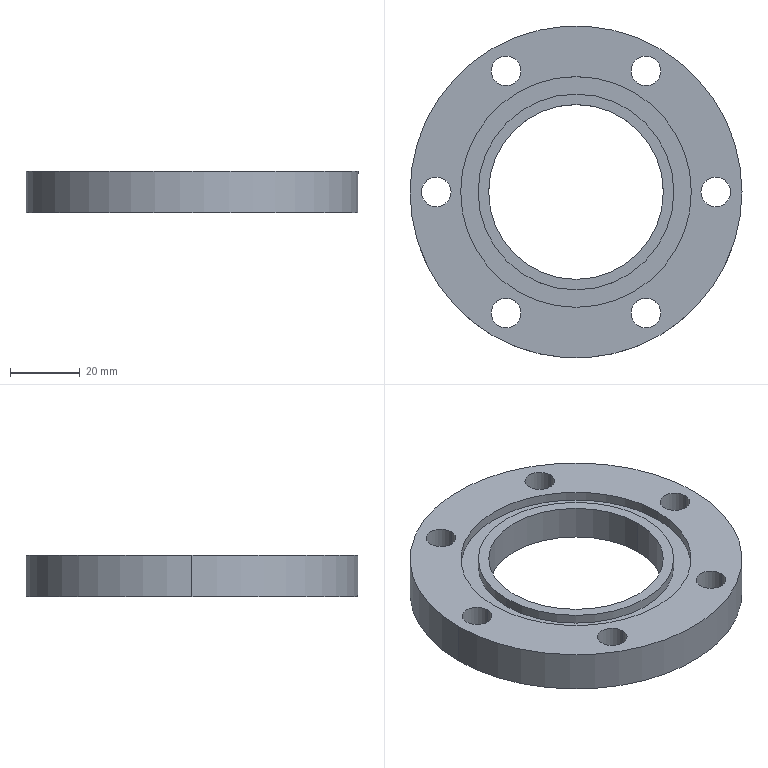Part | SolidWorks | features ICE 2, CirPattern 1, FlatPattern 1, HoleWzd 1, SMBaseFlange 1, SheetMetal 1 | 1 solid | 27 faces | box 95 x 95 x 12 mm | volume 53096 mm3 | cylinder 22 | plane 5 | commonest cylinder face diameters 8.5 x12 50 x2 56 x2 60 x2 66 x2 95 x2
STEP:
#1=CARTESIAN_POINT('',(15.75,-34.641,-12.));
#2=VERTEX_POINT('',#1);
#3=CARTESIAN_POINT('',(24.25,-34.641,-12.));
#4=VERTEX_POINT('',#3);
#5=CARTESIAN_POINT('',(20.,-34.641,-12.));
#6=DIRECTION('',(0.,0.,1.));
#7=DIRECTION('',(1.,0.,0.));
#8=AXIS2_PLACEMENT_3D('',#5,#6,#7);
#9=CIRCLE('',#8,4.25);
#10=EDGE_CURVE('',#2,#4,#9,.T.);
#11=ORIENTED_EDGE('',*,*,#10,.F.);
#12=CARTESIAN_POINT('',(15.75,-34.641,0.));
#13=VERTEX_POINT('',#12);
#14=CARTESIAN_POINT('',(15.75,-34.641,0.));
#15=DIRECTION('',(0.,0.,1.));
#16=VECTOR('',#15,1000.);
#17=LINE('',#14,#16);
#18=EDGE_CURVE('',#2,#13,#17,.T.);
#19=ORIENTED_EDGE('',*,*,#18,.T.);
#20=CARTESIAN_POINT('',(24.25,-34.641,0.));
#21=VERTEX_POINT('',#20);
#22=CARTESIAN_POINT('',(20.,-34.641,0.));
#23=DIRECTION('',(0.,0.,1.));
#24=DIRECTION('',(1.,0.,0.));
#25=AXIS2_PLACEMENT_3D('',#22,#23,#24);
#26=CIRCLE('',#25,4.25);
#27=EDGE_CURVE('',#13,#21,#26,.T.);
#28=ORIENTED_EDGE('',*,*,#27,.T.);
#29=CARTESIAN_POINT('',(24.25,-34.641,0.));
#30=DIRECTION('',(0.,0.,1.));
#31=VECTOR('',#30,1000.);
#32=LINE('',#29,#31);
#33=EDGE_CURVE('',#4,#21,#32,.T.);
#34=ORIENTED_EDGE('',*,*,#33,.F.);
#35=EDGE_LOOP('',(#11,#19,#28,#34));
#36=FACE_OUTER_BOUND('',#35,.T.);
#37=CARTESIAN_POINT('',(20.,-34.641,0.));
#38=DIRECTION('',(0.,0.,1.));
#39=DIRECTION('',(1.,0.,0.));
#40=AXIS2_PLACEMENT_3D('',#37,#38,#39);
#41=CYLINDRICAL_SURFACE('',#40,4.25);
#42=ADVANCED_FACE('',(#36),#41,.F.);
#43=CARTESIAN_POINT('',(-24.25,-34.641,-12.));
#44=VERTEX_POINT('',#43);
#45=CARTESIAN_POINT('',(-15.75,-34.641,-12.));
#46=VERTEX_POINT('',#45);
#47=CARTESIAN_POINT('',(-20.,-34.641,-12.));
#48=DIRECTION('',(0.,0.,1.));
#49=DIRECTION('',(1.,0.,0.));
#50=AXIS2_PLACEMENT_3D('',#47,#48,#49);
#51=CIRCLE('',#50,4.25);
#52=EDGE_CURVE('',#44,#46,#51,.T.);
#53=ORIENTED_EDGE('',*,*,#52,.F.);
#54=CARTESIAN_POINT('',(-24.25,-34.641,0.));
#55=VERTEX_POINT('',#54);
#56=CARTESIAN_POINT('',(-24.25,-34.641,0.));
#57=DIRECTION('',(0.,0.,1.));
#58=VECTOR('',#57,1000.);
#59=LINE('',#56,#58);
#60=EDGE_CURVE('',#44,#55,#59,.T.);
#61=ORIENTED_EDGE('',*,*,#60,.T.);
#62=CARTESIAN_POINT('',(-15.75,-34.641,0.));
#63=VERTEX_POINT('',#62);
#64=CARTESIAN_POINT('',(-20.,-34.641,0.));
#65=DIRECTION('',(0.,0.,1.));
#66=DIRECTION('',(1.,0.,0.));
#67=AXIS2_PLACEMENT_3D('',#64,#65,#66);
#68=CIRCLE('',#67,4.25);
#69=EDGE_CURVE('',#55,#63,#68,.T.);
#70=ORIENTED_EDGE('',*,*,#69,.T.);
#71=CARTESIAN_POINT('',(-15.75,-34.641,0.));
#72=DIRECTION('',(0.,0.,1.));
#73=VECTOR('',#72,1000.);
#74=LINE('',#71,#73);
#75=EDGE_CURVE('',#46,#63,#74,.T.);
#76=ORIENTED_EDGE('',*,*,#75,.F.);
#77=EDGE_LOOP('',(#53,#61,#70,#76));
#78=FACE_OUTER_BOUND('',#77,.T.);
#79=CARTESIAN_POINT('',(-20.,-34.641,0.));
#80=DIRECTION('',(0.,0.,1.));
#81=DIRECTION('',(1.,0.,0.));
#82=AXIS2_PLACEMENT_3D('',#79,#80,#81);
#83=CYLINDRICAL_SURFACE('',#82,4.25);
#84=ADVANCED_FACE('',(#78),#83,.F.);
#85=CARTESIAN_POINT('',(-44.25,0.,-12.));
#86=VERTEX_POINT('',#85);
#87=CARTESIAN_POINT('',(-35.75,0.,-12.));
#88=VERTEX_POINT('',#87);
#89=CARTESIAN_POINT('',(-40.,0.,-12.));
#90=DIRECTION('',(0.,0.,1.));
#91=DIRECTION('',(1.,0.,0.));
#92=AXIS2_PLACEMENT_3D('',#89,#90,#91);
#93=CIRCLE('',#92,4.25);
#94=EDGE_CURVE('',#86,#88,#93,.T.);
#95=ORIENTED_EDGE('',*,*,#94,.F.);
#96=CARTESIAN_POINT('',(-44.25,0.,0.));
#97=VERTEX_POINT('',#96);
#98=CARTESIAN_POINT('',(-44.25,0.,0.));
#99=DIRECTION('',(0.,0.,1.));
#100=VECTOR('',#99,1000.);
#101=LINE('',#98,#100);
#102=EDGE_CURVE('',#86,#97,#101,.T.);
#103=ORIENTED_EDGE('',*,*,#102,.T.);
#104=CARTESIAN_POINT('',(-35.75,0.,0.));
#105=VERTEX_POINT('',#104);
#106=CARTESIAN_POINT('',(-40.,0.,0.));
#107=DIRECTION('',(0.,0.,1.));
#108=DIRECTION('',(1.,0.,0.));
#109=AXIS2_PLACEMENT_3D('',#106,#107,#108);
#110=CIRCLE('',#109,4.25);
#111=EDGE_CURVE('',#97,#105,#110,.T.);
#112=ORIENTED_EDGE('',*,*,#111,.T.);
#113=CARTESIAN_POINT('',(-35.75,0.,0.));
#114=DIRECTION('',(0.,0.,1.));
#115=VECTOR('',#114,1000.);
#116=LINE('',#113,#115);
#117=EDGE_CURVE('',#88,#105,#116,.T.);
#118=ORIENTED_EDGE('',*,*,#117,.F.);
#119=EDGE_LOOP('',(#95,#103,#112,#118));
#120=FACE_OUTER_BOUND('',#119,.T.);
#121=CARTESIAN_POINT('',(-40.,0.,0.));
#122=DIRECTION('',(0.,0.,1.));
#123=DIRECTION('',(1.,0.,0.));
#124=AXIS2_PLACEMENT_3D('',#121,#122,#123);
#125=CYLINDRICAL_SURFACE('',#124,4.25);
#126=ADVANCED_FACE('',(#120),#125,.F.);
#127=CARTESIAN_POINT('',(-24.25,34.641,-12.));
#128=VERTEX_POINT('',#127);
#129=CARTESIAN_POINT('',(-15.75,34.641,-12.));
#130=VERTEX_POINT('',#129);
#131=CARTESIAN_POINT('',(-20.,34.641,-12.));
#132=DIRECTION('',(0.,0.,1.));
#133=DIRECTION('',(1.,0.,0.));
#134=AXIS2_PLACEMENT_3D('',#131,#132,#133);
#135=CIRCLE('',#134,4.25);
#136=EDGE_CURVE('',#128,#130,#135,.T.);
#137=ORIENTED_EDGE('',*,*,#136,.F.);
#138=CARTESIAN_POINT('',(-24.25,34.641,0.));
#139=VERTEX_POINT('',#138);
#140=CARTESIAN_POINT('',(-24.25,34.641,0.));
#141=DIRECTION('',(0.,0.,1.));
#142=VECTOR('',#141,1000.);
#143=LINE('',#140,#142);
#144=EDGE_CURVE('',#128,#139,#143,.T.);
#145=ORIENTED_EDGE('',*,*,#144,.T.);
#146=CARTESIAN_POINT('',(-15.75,34.641,0.));
#147=VERTEX_POINT('',#146);
#148=CARTESIAN_POINT('',(-20.,34.641,0.));
#149=DIRECTION('',(0.,0.,1.));
#150=DIRECTION('',(1.,0.,0.));
#151=AXIS2_PLACEMENT_3D('',#148,#149,#150);
#152=CIRCLE('',#151,4.25);
#153=EDGE_CURVE('',#139,#147,#152,.T.);
#154=ORIENTED_EDGE('',*,*,#153,.T.);
#155=CARTESIAN_POINT('',(-15.75,34.641,0.));
#156=DIRECTION('',(0.,0.,1.));
#157=VECTOR('',#156,1000.);
#158=LINE('',#155,#157);
#159=EDGE_CURVE('',#130,#147,#158,.T.);
#160=ORIENTED_EDGE('',*,*,#159,.F.);
#161=EDGE_LOOP('',(#137,#145,#154,#160));
#162=FACE_OUTER_BOUND('',#161,.T.);
#163=CARTESIAN_POINT('',(-20.,34.641,0.));
#164=DIRECTION('',(0.,0.,1.));
#165=DIRECTION('',(1.,0.,0.));
#166=AXIS2_PLACEMENT_3D('',#163,#164,#165);
#167=CYLINDRICAL_SURFACE('',#166,4.25);
#168=ADVANCED_FACE('',(#162),#167,.F.);
#169=CARTESIAN_POINT('',(15.75,34.641,-12.));
#170=VERTEX_POINT('',#169);
#171=CARTESIAN_POINT('',(24.25,34.641,-12.));
#172=VERTEX_POINT('',#171);
#173=CARTESIAN_POINT('',(20.,34.641,-12.));
#174=DIRECTION('',(0.,0.,1.));
#175=DIRECTION('',(1.,0.,0.));
#176=AXIS2_PLACEMENT_3D('',#173,#174,#175);
#177=CIRCLE('',#176,4.25);
#178=EDGE_CURVE('',#170,#172,#177,.T.);
#179=ORIENTED_EDGE('',*,*,#178,.F.);
#180=CARTESIAN_POINT('',(15.75,34.641,0.));
#181=VERTEX_POINT('',#180);
#182=CARTESIAN_POINT('',(15.75,34.641,0.));
#183=DIRECTION('',(0.,0.,1.));
#184=VECTOR('',#183,1000.);
#185=LINE('',#182,#184);
#186=EDGE_CURVE('',#170,#181,#185,.T.);
#187=ORIENTED_EDGE('',*,*,#186,.T.);
#188=CARTESIAN_POINT('',(24.25,34.641,0.));
#189=VERTEX_POINT('',#188);
#190=CARTESIAN_POINT('',(20.,34.641,0.));
#191=DIRECTION('',(0.,0.,1.));
#192=DIRECTION('',(1.,0.,0.));
#193=AXIS2_PLACEMENT_3D('',#190,#191,#192);
#194=CIRCLE('',#193,4.25);
#195=EDGE_CURVE('',#181,#189,#194,.T.);
#196=ORIENTED_EDGE('',*,*,#195,.T.);
#197=CARTESIAN_POINT('',(24.25,34.641,0.));
#198=DIRECTION('',(0.,0.,1.));
#199=VECTOR('',#198,1000.);
#200=LINE('',#197,#199);
#201=EDGE_CURVE('',#172,#189,#200,.T.);
#202=ORIENTED_EDGE('',*,*,#201,.F.);
#203=EDGE_LOOP('',(#179,#187,#196,#202));
#204=FACE_OUTER_BOUND('',#203,.T.);
#205=CARTESIAN_POINT('',(20.,34.641,0.));
#206=DIRECTION('',(0.,0.,1.));
#207=DIRECTION('',(1.,0.,0.));
#208=AXIS2_PLACEMENT_3D('',#205,#206,#207);
#209=CYLINDRICAL_SURFACE('',#208,4.25);
#210=ADVANCED_FACE('',(#204),#209,.F.);
#211=CARTESIAN_POINT('',(35.75,0.,-12.));
#212=VERTEX_POINT('',#211);
#213=CARTESIAN_POINT('',(44.25,0.,-12.));
#214=VERTEX_POINT('',#213);
#215=CARTESIAN_POINT('',(40.,0.,-12.));
#216=DIRECTION('',(0.,0.,1.));
#217=DIRECTION('',(1.,0.,0.));
#218=AXIS2_PLACEMENT_3D('',#215,#216,#217);
#219=CIRCLE('',#218,4.25);
#220=EDGE_CURVE('',#212,#214,#219,.T.);
#221=ORIENTED_EDGE('',*,*,#220,.F.);
#222=CARTESIAN_POINT('',(35.75,0.,0.));
#223=VERTEX_POINT('',#222);
#224=CARTESIAN_POINT('',(35.75,0.,0.));
#225=DIRECTION('',(0.,0.,1.));
#226=VECTOR('',#225,1000.);
#227=LINE('',#224,#226);
#228=EDGE_CURVE('',#212,#223,#227,.T.);
#229=ORIENTED_EDGE('',*,*,#228,.T.);
#230=CARTESIAN_POINT('',(44.25,0.,0.));
#231=VERTEX_POINT('',#230);
#232=CARTESIAN_POINT('',(40.,0.,0.));
#233=DIRECTION('',(0.,0.,1.));
#234=DIRECTION('',(1.,0.,0.));
#235=AXIS2_PLACEMENT_3D('',#232,#233,#234);
#236=CIRCLE('',#235,4.25);
#237=EDGE_CURVE('',#223,#231,#236,.T.);
#238=ORIENTED_EDGE('',*,*,#237,.T.);
#239=CARTESIAN_POINT('',(44.25,0.,0.));
#240=DIRECTION('',(0.,0.,1.));
#241=VECTOR('',#240,1000.);
#242=LINE('',#239,#241);
#243=EDGE_CURVE('',#214,#231,#242,.T.);
#244=ORIENTED_EDGE('',*,*,#243,.F.);
#245=EDGE_LOOP('',(#221,#229,#238,#244));
#246=FACE_OUTER_BOUND('',#245,.T.);
#247=CARTESIAN_POINT('',(40.,0.,0.));
#248=DIRECTION('',(0.,0.,1.));
#249=DIRECTION('',(1.,0.,0.));
#250=AXIS2_PLACEMENT_3D('',#247,#248,#249);
#251=CYLINDRICAL_SURFACE('',#250,4.25);
#252=ADVANCED_FACE('',(#246),#251,.F.);
#253=CARTESIAN_POINT('',(30.,0.,-12.));
#254=VERTEX_POINT('',#253);
#255=CARTESIAN_POINT('',(-30.,0.,-12.));
#256=VERTEX_POINT('',#255);
#257=CARTESIAN_POINT('',(0.,0.,-12.));
#258=DIRECTION('',(0.,0.,-1.));
#259=DIRECTION('',(-1.,0.,0.));
#260=AXIS2_PLACEMENT_3D('',#257,#258,#259);
#261=CIRCLE('',#260,30.);
#262=EDGE_CURVE('',#254,#256,#261,.T.);
#263=ORIENTED_EDGE('',*,*,#262,.T.);
#264=CARTESIAN_POINT('',(-30.,0.,-10.));
#265=VERTEX_POINT('',#264);
#266=CARTESIAN_POINT('',(-30.,0.,-12.));
#267=DIRECTION('',(0.,0.,1.));
#268=VECTOR('',#267,1000.);
#269=LINE('',#266,#268);
#270=EDGE_CURVE('',#256,#265,#269,.T.);
#271=ORIENTED_EDGE('',*,*,#270,.T.);
#272=CARTESIAN_POINT('',(30.,0.,-10.));
#273=VERTEX_POINT('',#272);
#274=CARTESIAN_POINT('',(0.,0.,-10.));
#275=DIRECTION('',(0.,0.,-1.));
#276=DIRECTION('',(-1.,0.,0.));
#277=AXIS2_PLACEMENT_3D('',#274,#275,#276);
#278=CIRCLE('',#277,30.);
#279=EDGE_CURVE('',#273,#265,#278,.T.);
#280=ORIENTED_EDGE('',*,*,#279,.F.);
#281=CARTESIAN_POINT('',(30.,0.,-12.));
#282=DIRECTION('',(0.,0.,1.));
#283=VECTOR('',#282,1000.);
#284=LINE('',#281,#283);
#285=EDGE_CURVE('',#254,#273,#284,.T.);
#286=ORIENTED_EDGE('',*,*,#285,.F.);
#287=EDGE_LOOP('',(#263,#271,#280,#286));
#288=FACE_OUTER_BOUND('',#287,.T.);
#289=CARTESIAN_POINT('',(0.,0.,-12.));
#290=DIRECTION('',(0.,0.,1.));
#291=DIRECTION('',(1.,0.,0.));
#292=AXIS2_PLACEMENT_3D('',#289,#290,#291);
#293=CYLINDRICAL_SURFACE('',#292,30.);
#294=ADVANCED_FACE('',(#288),#293,.F.);
#295=CARTESIAN_POINT('',(28.,0.,-2.7));
#296=VERTEX_POINT('',#295);
#297=CARTESIAN_POINT('',(-28.,0.,-2.7));
#298=VERTEX_POINT('',#297);
#299=CARTESIAN_POINT('',(0.,0.,-2.7));
#300=DIRECTION('',(0.,0.,1.));
#301=DIRECTION('',(1.,0.,0.));
#302=AXIS2_PLACEMENT_3D('',#299,#300,#301);
#303=CIRCLE('',#302,28.);
#304=EDGE_CURVE('',#296,#298,#303,.T.);
#305=ORIENTED_EDGE('',*,*,#304,.T.);
#306=CARTESIAN_POINT('',(-28.,0.,0.));
#307=VERTEX_POINT('',#306);
#308=CARTESIAN_POINT('',(-28.,0.,-2.7));
#309=DIRECTION('',(0.,0.,1.));
#310=VECTOR('',#309,1000.);
#311=LINE('',#308,#310);
#312=EDGE_CURVE('',#298,#307,#311,.T.);
#313=ORIENTED_EDGE('',*,*,#312,.T.);
#314=CARTESIAN_POINT('',(28.,0.,0.));
#315=VERTEX_POINT('',#314);
#316=CARTESIAN_POINT('',(0.,0.,0.));
#317=DIRECTION('',(0.,0.,1.));
#318=DIRECTION('',(1.,0.,0.));
#319=AXIS2_PLACEMENT_3D('',#316,#317,#318);
#320=CIRCLE('',#319,28.);
#321=EDGE_CURVE('',#315,#307,#320,.T.);
#322=ORIENTED_EDGE('',*,*,#321,.F.);
#323=CARTESIAN_POINT('',(28.,0.,-2.7));
#324=DIRECTION('',(0.,0.,1.));
#325=VECTOR('',#324,1000.);
#326=LINE('',#323,#325);
#327=EDGE_CURVE('',#296,#315,#326,.T.);
#328=ORIENTED_EDGE('',*,*,#327,.F.);
#329=EDGE_LOOP('',(#305,#313,#322,#328));
#330=FACE_OUTER_BOUND('',#329,.T.);
#331=CARTESIAN_POINT('',(0.,0.,-2.7));
#332=DIRECTION('',(0.,0.,1.));
#333=DIRECTION('',(1.,0.,0.));
#334=AXIS2_PLACEMENT_3D('',#331,#332,#333);
#335=CYLINDRICAL_SURFACE('',#334,28.);
#336=ADVANCED_FACE('',(#330),#335,.T.);
#337=CARTESIAN_POINT('',(-33.,0.,-2.7));
#338=VERTEX_POINT('',#337);
#339=CARTESIAN_POINT('',(33.,0.,-2.7));
#340=VERTEX_POINT('',#339);
#341=CARTESIAN_POINT('',(0.,0.,-2.7));
#342=DIRECTION('',(0.,0.,1.));
#343=DIRECTION('',(1.,0.,0.));
#344=AXIS2_PLACEMENT_3D('',#341,#342,#343);
#345=CIRCLE('',#344,33.);
#346=EDGE_CURVE('',#338,#340,#345,.T.);
#347=ORIENTED_EDGE('',*,*,#346,.F.);
#348=CARTESIAN_POINT('',(-33.,0.,0.));
#349=VERTEX_POINT('',#348);
#350=CARTESIAN_POINT('',(-33.,0.,-2.7));
#351=DIRECTION('',(0.,0.,1.));
#352=VECTOR('',#351,1000.);
#353=LINE('',#350,#352);
#354=EDGE_CURVE('',#338,#349,#353,.T.);
#355=ORIENTED_EDGE('',*,*,#354,.T.);
#356=CARTESIAN_POINT('',(33.,0.,0.));
#357=VERTEX_POINT('',#356);
#358=CARTESIAN_POINT('',(0.,0.,0.));
#359=DIRECTION('',(0.,0.,1.));
#360=DIRECTION('',(1.,0.,0.));
#361=AXIS2_PLACEMENT_3D('',#358,#359,#360);
#362=CIRCLE('',#361,33.);
#363=EDGE_CURVE('',#349,#357,#362,.T.);
#364=ORIENTED_EDGE('',*,*,#363,.T.);
#365=CARTESIAN_POINT('',(33.,0.,-2.7));
#366=DIRECTION('',(0.,0.,1.));
#367=VECTOR('',#366,1000.);
#368=LINE('',#365,#367);
#369=EDGE_CURVE('',#340,#357,#368,.T.);
#370=ORIENTED_EDGE('',*,*,#369,.F.);
#371=EDGE_LOOP('',(#347,#355,#364,#370));
#372=FACE_OUTER_BOUND('',#371,.T.);
#373=CARTESIAN_POINT('',(0.,0.,-2.7));
#374=DIRECTION('',(0.,0.,1.));
#375=DIRECTION('',(1.,0.,0.));
#376=AXIS2_PLACEMENT_3D('',#373,#374,#375);
#377=CYLINDRICAL_SURFACE('',#376,33.);
#378=ADVANCED_FACE('',(#372),#377,.F.);
#379=CARTESIAN_POINT('',(-25.,0.,-10.));
#380=VERTEX_POINT('',#379);
#381=CARTESIAN_POINT('',(25.,0.,-10.));
#382=VERTEX_POINT('',#381);
#383=CARTESIAN_POINT('',(0.,0.,-10.));
#384=DIRECTION('',(0.,0.,1.));
#385=DIRECTION('',(1.,0.,0.));
#386=AXIS2_PLACEMENT_3D('',#383,#384,#385);
#387=CIRCLE('',#386,25.);
#388=EDGE_CURVE('',#380,#382,#387,.T.);
#389=ORIENTED_EDGE('',*,*,#388,.F.);
#390=CARTESIAN_POINT('',(-25.,0.,0.));
#391=VERTEX_POINT('',#390);
#392=CARTESIAN_POINT('',(-25.,0.,-10.));
#393=DIRECTION('',(0.,0.,1.));
#394=VECTOR('',#393,1000.);
#395=LINE('',#392,#394);
#396=EDGE_CURVE('',#380,#391,#395,.T.);
#397=ORIENTED_EDGE('',*,*,#396,.T.);
#398=CARTESIAN_POINT('',(25.,0.,0.));
#399=VERTEX_POINT('',#398);
#400=CARTESIAN_POINT('',(0.,0.,0.));
#401=DIRECTION('',(0.,0.,1.));
#402=DIRECTION('',(1.,0.,0.));
#403=AXIS2_PLACEMENT_3D('',#400,#401,#402);
#404=CIRCLE('',#403,25.);
#405=EDGE_CURVE('',#391,#399,#404,.T.);
#406=ORIENTED_EDGE('',*,*,#405,.T.);
#407=CARTESIAN_POINT('',(25.,0.,-10.));
#408=DIRECTION('',(0.,0.,1.));
#409=VECTOR('',#408,1000.);
#410=LINE('',#407,#409);
#411=EDGE_CURVE('',#382,#399,#410,.T.);
#412=ORIENTED_EDGE('',*,*,#411,.F.);
#413=EDGE_LOOP('',(#389,#397,#406,#412));
#414=FACE_OUTER_BOUND('',#413,.T.);
#415=CARTESIAN_POINT('',(0.,0.,-10.));
#416=DIRECTION('',(0.,0.,1.));
#417=DIRECTION('',(1.,0.,0.));
#418=AXIS2_PLACEMENT_3D('',#415,#416,#417);
#419=CYLINDRICAL_SURFACE('',#418,25.);
#420=ADVANCED_FACE('',(#414),#419,.F.);
#421=CARTESIAN_POINT('',(-47.5,0.,-12.));
#422=VERTEX_POINT('',#421);
#423=CARTESIAN_POINT('',(47.5,0.,-12.));
#424=VERTEX_POINT('',#423);
#425=CARTESIAN_POINT('',(0.,0.,-12.));
#426=DIRECTION('',(0.,0.,-1.));
#427=DIRECTION('',(-1.,0.,0.));
#428=AXIS2_PLACEMENT_3D('',#425,#426,#427);
#429=CIRCLE('',#428,47.5);
#430=EDGE_CURVE('',#422,#424,#429,.T.);
#431=ORIENTED_EDGE('',*,*,#430,.F.);
#432=CARTESIAN_POINT('',(-47.5,0.,0.));
#433=VERTEX_POINT('',#432);
#434=CARTESIAN_POINT('',(-47.5,0.,-10.));
#435=DIRECTION('',(0.,0.,1.));
#436=VECTOR('',#435,1000.);
#437=LINE('',#434,#436);
#438=EDGE_CURVE('',#422,#433,#437,.T.);
#439=ORIENTED_EDGE('',*,*,#438,.T.);
#440=CARTESIAN_POINT('',(47.5,0.,0.));
#441=VERTEX_POINT('',#440);
#442=CARTESIAN_POINT('',(0.,0.,0.));
#443=DIRECTION('',(0.,0.,1.));
#444=DIRECTION('',(1.,0.,0.));
#445=AXIS2_PLACEMENT_3D('',#442,#443,#444);
#446=CIRCLE('',#445,47.5);
#447=EDGE_CURVE('',#441,#433,#446,.T.);
#448=ORIENTED_EDGE('',*,*,#447,.F.);
#449=CARTESIAN_POINT('',(47.5,0.,-10.));
#450=DIRECTION('',(0.,0.,1.));
#451=VECTOR('',#450,1000.);
#452=LINE('',#449,#451);
#453=EDGE_CURVE('',#424,#441,#452,.T.);
#454=ORIENTED_EDGE('',*,*,#453,.F.);
#455=EDGE_LOOP('',(#431,#439,#448,#454));
#456=FACE_OUTER_BOUND('',#455,.T.);
#457=CARTESIAN_POINT('',(0.,0.,-10.));
#458=DIRECTION('',(0.,0.,1.));
#459=DIRECTION('',(1.,0.,0.));
#460=AXIS2_PLACEMENT_3D('',#457,#458,#459);
#461=CYLINDRICAL_SURFACE('',#460,47.5);
#462=ADVANCED_FACE('',(#456),#461,.T.);
#463=CARTESIAN_POINT('',(0.,0.,-10.));
#464=DIRECTION('',(0.,0.,1.));
#465=DIRECTION('',(1.,0.,0.));
#466=AXIS2_PLACEMENT_3D('',#463,#464,#465);
#467=CIRCLE('',#466,25.);
#468=EDGE_CURVE('',#382,#380,#467,.T.);
#469=ORIENTED_EDGE('',*,*,#468,.T.);
#470=ORIENTED_EDGE('',*,*,#388,.T.);
#471=EDGE_LOOP('',(#469,#470));
#472=FACE_BOUND('',#471,.T.);
#473=ORIENTED_EDGE('',*,*,#279,.T.);
#474=CARTESIAN_POINT('',(0.,0.,-10.));
#475=DIRECTION('',(0.,0.,-1.));
#476=DIRECTION('',(-1.,0.,0.));
#477=AXIS2_PLACEMENT_3D('',#474,#475,#476);
#478=CIRCLE('',#477,30.);
#479=EDGE_CURVE('',#265,#273,#478,.T.);
#480=ORIENTED_EDGE('',*,*,#479,.T.);
#481=EDGE_LOOP('',(#473,#480));
#482=FACE_OUTER_BOUND('',#481,.T.);
#483=CARTESIAN_POINT('',(0.,0.,-10.));
#484=DIRECTION('',(0.,0.,1.));
#485=DIRECTION('',(1.,0.,0.));
#486=AXIS2_PLACEMENT_3D('',#483,#484,#485);
#487=PLANE('',#486);
#488=ADVANCED_FACE('',(#472,#482),#487,.F.);
#489=CARTESIAN_POINT('',(0.,0.,0.));
#490=DIRECTION('',(0.,0.,1.));
#491=DIRECTION('',(1.,0.,0.));
#492=AXIS2_PLACEMENT_3D('',#489,#490,#491);
#493=CIRCLE('',#492,25.);
#494=EDGE_CURVE('',#399,#391,#493,.T.);
#495=ORIENTED_EDGE('',*,*,#494,.F.);
#496=ORIENTED_EDGE('',*,*,#405,.F.);
#497=EDGE_LOOP('',(#495,#496));
#498=FACE_BOUND('',#497,.T.);
#499=ORIENTED_EDGE('',*,*,#321,.T.);
#500=CARTESIAN_POINT('',(0.,0.,0.));
#501=DIRECTION('',(0.,0.,1.));
#502=DIRECTION('',(1.,0.,0.));
#503=AXIS2_PLACEMENT_3D('',#500,#501,#502);
#504=CIRCLE('',#503,28.);
#505=EDGE_CURVE('',#307,#315,#504,.T.);
#506=ORIENTED_EDGE('',*,*,#505,.T.);
#507=EDGE_LOOP('',(#499,#506));
#508=FACE_OUTER_BOUND('',#507,.T.);
#509=CARTESIAN_POINT('',(0.,0.,0.));
#510=DIRECTION('',(0.,0.,1.));
#511=DIRECTION('',(1.,0.,0.));
#512=AXIS2_PLACEMENT_3D('',#509,#510,#511);
#513=PLANE('',#512);
#514=ADVANCED_FACE('',(#498,#508),#513,.T.);
#515=ORIENTED_EDGE('',*,*,#438,.F.);
#516=CARTESIAN_POINT('',(0.,0.,-12.));
#517=DIRECTION('',(0.,0.,-1.));
#518=DIRECTION('',(-1.,0.,0.));
#519=AXIS2_PLACEMENT_3D('',#516,#517,#518);
#520=CIRCLE('',#519,47.5);
#521=EDGE_CURVE('',#424,#422,#520,.T.);
#522=ORIENTED_EDGE('',*,*,#521,.F.);
#523=ORIENTED_EDGE('',*,*,#453,.T.);
#524=CARTESIAN_POINT('',(0.,0.,0.));
#525=DIRECTION('',(0.,0.,1.));
#526=DIRECTION('',(1.,0.,0.));
#527=AXIS2_PLACEMENT_3D('',#524,#525,#526);
#528=CIRCLE('',#527,47.5);
#529=EDGE_CURVE('',#433,#441,#528,.T.);
#530=ORIENTED_EDGE('',*,*,#529,.F.);
#531=EDGE_LOOP('',(#515,#522,#523,#530));
#532=FACE_OUTER_BOUND('',#531,.T.);
#533=CARTESIAN_POINT('',(0.,0.,-10.));
#534=DIRECTION('',(0.,0.,1.));
#535=DIRECTION('',(1.,0.,0.));
#536=AXIS2_PLACEMENT_3D('',#533,#534,#535);
#537=CYLINDRICAL_SURFACE('',#536,47.5);
#538=ADVANCED_FACE('',(#532),#537,.T.);
#539=CARTESIAN_POINT('',(20.,-34.641,0.));
#540=DIRECTION('',(0.,0.,1.));
#541=DIRECTION('',(1.,0.,0.));
#542=AXIS2_PLACEMENT_3D('',#539,#540,#541);
#543=CIRCLE('',#542,4.25);
#544=EDGE_CURVE('',#21,#13,#543,.T.);
#545=ORIENTED_EDGE('',*,*,#544,.F.);
#546=ORIENTED_EDGE('',*,*,#27,.F.);
#547=EDGE_LOOP('',(#545,#546));
#548=FACE_BOUND('',#547,.T.);
#549=CARTESIAN_POINT('',(-20.,-34.641,0.));
#550=DIRECTION('',(0.,0.,1.));
#551=DIRECTION('',(1.,0.,0.));
#552=AXIS2_PLACEMENT_3D('',#549,#550,#551);
#553=CIRCLE('',#552,4.25);
#554=EDGE_CURVE('',#63,#55,#553,.T.);
#555=ORIENTED_EDGE('',*,*,#554,.F.);
#556=ORIENTED_EDGE('',*,*,#69,.F.);
#557=EDGE_LOOP('',(#555,#556));
#558=FACE_BOUND('',#557,.T.);
#559=CARTESIAN_POINT('',(-40.,0.,0.));
#560=DIRECTION('',(0.,0.,1.));
#561=DIRECTION('',(1.,0.,0.));
#562=AXIS2_PLACEMENT_3D('',#559,#560,#561);
#563=CIRCLE('',#562,4.25);
#564=EDGE_CURVE('',#105,#97,#563,.T.);
#565=ORIENTED_EDGE('',*,*,#564,.F.);
#566=ORIENTED_EDGE('',*,*,#111,.F.);
#567=EDGE_LOOP('',(#565,#566));
#568=FACE_BOUND('',#567,.T.);
#569=CARTESIAN_POINT('',(-20.,34.641,0.));
#570=DIRECTION('',(0.,0.,1.));
#571=DIRECTION('',(1.,0.,0.));
#572=AXIS2_PLACEMENT_3D('',#569,#570,#571);
#573=CIRCLE('',#572,4.25);
#574=EDGE_CURVE('',#147,#139,#573,.T.);
#575=ORIENTED_EDGE('',*,*,#574,.F.);
#576=ORIENTED_EDGE('',*,*,#153,.F.);
#577=EDGE_LOOP('',(#575,#576));
#578=FACE_BOUND('',#577,.T.);
#579=CARTESIAN_POINT('',(20.,34.641,0.));
#580=DIRECTION('',(0.,0.,1.));
#581=DIRECTION('',(1.,0.,0.));
#582=AXIS2_PLACEMENT_3D('',#579,#580,#581);
#583=CIRCLE('',#582,4.25);
#584=EDGE_CURVE('',#189,#181,#583,.T.);
#585=ORIENTED_EDGE('',*,*,#584,.F.);
#586=ORIENTED_EDGE('',*,*,#195,.F.);
#587=EDGE_LOOP('',(#585,#586));
#588=FACE_BOUND('',#587,.T.);
#589=CARTESIAN_POINT('',(40.,0.,0.));
#590=DIRECTION('',(0.,0.,1.));
#591=DIRECTION('',(1.,0.,0.));
#592=AXIS2_PLACEMENT_3D('',#589,#590,#591);
#593=CIRCLE('',#592,4.25);
#594=EDGE_CURVE('',#231,#223,#593,.T.);
#595=ORIENTED_EDGE('',*,*,#594,.F.);
#596=ORIENTED_EDGE('',*,*,#237,.F.);
#597=EDGE_LOOP('',(#595,#596));
#598=FACE_BOUND('',#597,.T.);
#599=CARTESIAN_POINT('',(0.,0.,0.));
#600=DIRECTION('',(0.,0.,1.));
#601=DIRECTION('',(1.,0.,0.));
#602=AXIS2_PLACEMENT_3D('',#599,#600,#601);
#603=CIRCLE('',#602,33.);
#604=EDGE_CURVE('',#357,#349,#603,.T.);
#605=ORIENTED_EDGE('',*,*,#604,.F.);
#606=ORIENTED_EDGE('',*,*,#363,.F.);
#607=EDGE_LOOP('',(#605,#606));
#608=FACE_BOUND('',#607,.T.);
#609=ORIENTED_EDGE('',*,*,#447,.T.);
#610=ORIENTED_EDGE('',*,*,#529,.T.);
#611=EDGE_LOOP('',(#609,#610));
#612=FACE_OUTER_BOUND('',#611,.T.);
#613=CARTESIAN_POINT('',(0.,0.,0.));
#614=DIRECTION('',(0.,0.,1.));
#615=DIRECTION('',(1.,0.,0.));
#616=AXIS2_PLACEMENT_3D('',#613,#614,#615);
#617=PLANE('',#616);
#618=ADVANCED_FACE('',(#548,#558,#568,#578,#588,#598,#608,#612),#617,.T.);
#619=ORIENTED_EDGE('',*,*,#396,.F.);
#620=ORIENTED_EDGE('',*,*,#468,.F.);
#621=ORIENTED_EDGE('',*,*,#411,.T.);
#622=ORIENTED_EDGE('',*,*,#494,.T.);
#623=EDGE_LOOP('',(#619,#620,#621,#622));
#624=FACE_OUTER_BOUND('',#623,.T.);
#625=CARTESIAN_POINT('',(0.,0.,-10.));
#626=DIRECTION('',(0.,0.,1.));
#627=DIRECTION('',(1.,0.,0.));
#628=AXIS2_PLACEMENT_3D('',#625,#626,#627);
#629=CYLINDRICAL_SURFACE('',#628,25.);
#630=ADVANCED_FACE('',(#624),#629,.F.);
#631=ORIENTED_EDGE('',*,*,#354,.F.);
#632=CARTESIAN_POINT('',(0.,0.,-2.7));
#633=DIRECTION('',(0.,0.,1.));
#634=DIRECTION('',(1.,0.,0.));
#635=AXIS2_PLACEMENT_3D('',#632,#633,#634);
#636=CIRCLE('',#635,33.);
#637=EDGE_CURVE('',#340,#338,#636,.T.);
#638=ORIENTED_EDGE('',*,*,#637,.F.);
#639=ORIENTED_EDGE('',*,*,#369,.T.);
#640=ORIENTED_EDGE('',*,*,#604,.T.);
#641=EDGE_LOOP('',(#631,#638,#639,#640));
#642=FACE_OUTER_BOUND('',#641,.T.);
#643=CARTESIAN_POINT('',(0.,0.,-2.7));
#644=DIRECTION('',(0.,0.,1.));
#645=DIRECTION('',(1.,0.,0.));
#646=AXIS2_PLACEMENT_3D('',#643,#644,#645);
#647=CYLINDRICAL_SURFACE('',#646,33.);
#648=ADVANCED_FACE('',(#642),#647,.F.);
#649=ORIENTED_EDGE('',*,*,#304,.F.);
#650=CARTESIAN_POINT('',(0.,0.,-2.7));
#651=DIRECTION('',(0.,0.,1.));
#652=DIRECTION('',(1.,0.,0.));
#653=AXIS2_PLACEMENT_3D('',#650,#651,#652);
#654=CIRCLE('',#653,28.);
#655=EDGE_CURVE('',#298,#296,#654,.T.);
#656=ORIENTED_EDGE('',*,*,#655,.F.);
#657=EDGE_LOOP('',(#649,#656));
#658=FACE_BOUND('',#657,.T.);
#659=ORIENTED_EDGE('',*,*,#637,.T.);
#660=ORIENTED_EDGE('',*,*,#346,.T.);
#661=EDGE_LOOP('',(#659,#660));
#662=FACE_OUTER_BOUND('',#661,.T.);
#663=CARTESIAN_POINT('',(0.,0.,-2.7));
#664=DIRECTION('',(0.,0.,1.));
#665=DIRECTION('',(1.,0.,0.));
#666=AXIS2_PLACEMENT_3D('',#663,#664,#665);
#667=PLANE('',#666);
#668=ADVANCED_FACE('',(#658,#662),#667,.T.);
#669=ORIENTED_EDGE('',*,*,#312,.F.);
#670=ORIENTED_EDGE('',*,*,#655,.T.);
#671=ORIENTED_EDGE('',*,*,#327,.T.);
#672=ORIENTED_EDGE('',*,*,#505,.F.);
#673=EDGE_LOOP('',(#669,#670,#671,#672));
#674=FACE_OUTER_BOUND('',#673,.T.);
#675=CARTESIAN_POINT('',(0.,0.,-2.7));
#676=DIRECTION('',(0.,0.,1.));
#677=DIRECTION('',(1.,0.,0.));
#678=AXIS2_PLACEMENT_3D('',#675,#676,#677);
#679=CYLINDRICAL_SURFACE('',#678,28.);
#680=ADVANCED_FACE('',(#674),#679,.T.);
#681=CARTESIAN_POINT('',(20.,-34.641,-12.));
#682=DIRECTION('',(0.,0.,1.));
#683=DIRECTION('',(1.,0.,0.));
#684=AXIS2_PLACEMENT_3D('',#681,#682,#683);
#685=CIRCLE('',#684,4.25);
#686=EDGE_CURVE('',#4,#2,#685,.T.);
#687=ORIENTED_EDGE('',*,*,#686,.T.);
#688=ORIENTED_EDGE('',*,*,#10,.T.);
#689=EDGE_LOOP('',(#687,#688));
#690=FACE_BOUND('',#689,.T.);
#691=CARTESIAN_POINT('',(-20.,-34.641,-12.));
#692=DIRECTION('',(0.,0.,1.));
#693=DIRECTION('',(1.,0.,0.));
#694=AXIS2_PLACEMENT_3D('',#691,#692,#693);
#695=CIRCLE('',#694,4.25);
#696=EDGE_CURVE('',#46,#44,#695,.T.);
#697=ORIENTED_EDGE('',*,*,#696,.T.);
#698=ORIENTED_EDGE('',*,*,#52,.T.);
#699=EDGE_LOOP('',(#697,#698));
#700=FACE_BOUND('',#699,.T.);
#701=CARTESIAN_POINT('',(-40.,0.,-12.));
#702=DIRECTION('',(0.,0.,1.));
#703=DIRECTION('',(1.,0.,0.));
#704=AXIS2_PLACEMENT_3D('',#701,#702,#703);
#705=CIRCLE('',#704,4.25);
#706=EDGE_CURVE('',#88,#86,#705,.T.);
#707=ORIENTED_EDGE('',*,*,#706,.T.);
#708=ORIENTED_EDGE('',*,*,#94,.T.);
#709=EDGE_LOOP('',(#707,#708));
#710=FACE_BOUND('',#709,.T.);
#711=CARTESIAN_POINT('',(-20.,34.641,-12.));
#712=DIRECTION('',(0.,0.,1.));
#713=DIRECTION('',(1.,0.,0.));
#714=AXIS2_PLACEMENT_3D('',#711,#712,#713);
#715=CIRCLE('',#714,4.25);
#716=EDGE_CURVE('',#130,#128,#715,.T.);
#717=ORIENTED_EDGE('',*,*,#716,.T.);
#718=ORIENTED_EDGE('',*,*,#136,.T.);
#719=EDGE_LOOP('',(#717,#718));
#720=FACE_BOUND('',#719,.T.);
#721=CARTESIAN_POINT('',(20.,34.641,-12.));
#722=DIRECTION('',(0.,0.,1.));
#723=DIRECTION('',(1.,0.,0.));
#724=AXIS2_PLACEMENT_3D('',#721,#722,#723);
#725=CIRCLE('',#724,4.25);
#726=EDGE_CURVE('',#172,#170,#725,.T.);
#727=ORIENTED_EDGE('',*,*,#726,.T.);
#728=ORIENTED_EDGE('',*,*,#178,.T.);
#729=EDGE_LOOP('',(#727,#728));
#730=FACE_BOUND('',#729,.T.);
#731=CARTESIAN_POINT('',(40.,0.,-12.));
#732=DIRECTION('',(0.,0.,1.));
#733=DIRECTION('',(1.,0.,0.));
#734=AXIS2_PLACEMENT_3D('',#731,#732,#733);
#735=CIRCLE('',#734,4.25);
#736=EDGE_CURVE('',#214,#212,#735,.T.);
#737=ORIENTED_EDGE('',*,*,#736,.T.);
#738=ORIENTED_EDGE('',*,*,#220,.T.);
#739=EDGE_LOOP('',(#737,#738));
#740=FACE_BOUND('',#739,.T.);
#741=ORIENTED_EDGE('',*,*,#521,.T.);
#742=ORIENTED_EDGE('',*,*,#430,.T.);
#743=EDGE_LOOP('',(#741,#742));
#744=FACE_OUTER_BOUND('',#743,.T.);
#745=ORIENTED_EDGE('',*,*,#262,.F.);
#746=CARTESIAN_POINT('',(0.,0.,-12.));
#747=DIRECTION('',(0.,0.,-1.));
#748=DIRECTION('',(-1.,0.,0.));
#749=AXIS2_PLACEMENT_3D('',#746,#747,#748);
#750=CIRCLE('',#749,30.);
#751=EDGE_CURVE('',#256,#254,#750,.T.);
#752=ORIENTED_EDGE('',*,*,#751,.F.);
#753=EDGE_LOOP('',(#745,#752));
#754=FACE_BOUND('',#753,.T.);
#755=CARTESIAN_POINT('',(0.,0.,-12.));
#756=DIRECTION('',(0.,0.,-1.));
#757=DIRECTION('',(-1.,0.,0.));
#758=AXIS2_PLACEMENT_3D('',#755,#756,#757);
#759=PLANE('',#758);
#760=ADVANCED_FACE('',(#690,#700,#710,#720,#730,#740,#744,#754),#759,.T.);
#761=ORIENTED_EDGE('',*,*,#270,.F.);
#762=ORIENTED_EDGE('',*,*,#751,.T.);
#763=ORIENTED_EDGE('',*,*,#285,.T.);
#764=ORIENTED_EDGE('',*,*,#479,.F.);
#765=EDGE_LOOP('',(#761,#762,#763,#764));
#766=FACE_OUTER_BOUND('',#765,.T.);
#767=CARTESIAN_POINT('',(0.,0.,-12.));
#768=DIRECTION('',(0.,0.,1.));
#769=DIRECTION('',(1.,0.,0.));
#770=AXIS2_PLACEMENT_3D('',#767,#768,#769);
#771=CYLINDRICAL_SURFACE('',#770,30.);
#772=ADVANCED_FACE('',(#766),#771,.F.);
#773=ORIENTED_EDGE('',*,*,#228,.F.);
#774=ORIENTED_EDGE('',*,*,#736,.F.);
#775=ORIENTED_EDGE('',*,*,#243,.T.);
#776=ORIENTED_EDGE('',*,*,#594,.T.);
#777=EDGE_LOOP('',(#773,#774,#775,#776));
#778=FACE_OUTER_BOUND('',#777,.T.);
#779=CARTESIAN_POINT('',(40.,0.,0.));
#780=DIRECTION('',(0.,0.,1.));
#781=DIRECTION('',(1.,0.,0.));
#782=AXIS2_PLACEMENT_3D('',#779,#780,#781);
#783=CYLINDRICAL_SURFACE('',#782,4.25);
#784=ADVANCED_FACE('',(#778),#783,.F.);
#785=ORIENTED_EDGE('',*,*,#186,.F.);
#786=ORIENTED_EDGE('',*,*,#726,.F.);
#787=ORIENTED_EDGE('',*,*,#201,.T.);
#788=ORIENTED_EDGE('',*,*,#584,.T.);
#789=EDGE_LOOP('',(#785,#786,#787,#788));
#790=FACE_OUTER_BOUND('',#789,.T.);
#791=CARTESIAN_POINT('',(20.,34.641,0.));
#792=DIRECTION('',(0.,0.,1.));
#793=DIRECTION('',(1.,0.,0.));
#794=AXIS2_PLACEMENT_3D('',#791,#792,#793);
#795=CYLINDRICAL_SURFACE('',#794,4.25);
#796=ADVANCED_FACE('',(#790),#795,.F.);
#797=ORIENTED_EDGE('',*,*,#144,.F.);
#798=ORIENTED_EDGE('',*,*,#716,.F.);
#799=ORIENTED_EDGE('',*,*,#159,.T.);
#800=ORIENTED_EDGE('',*,*,#574,.T.);
#801=EDGE_LOOP('',(#797,#798,#799,#800));
#802=FACE_OUTER_BOUND('',#801,.T.);
#803=CARTESIAN_POINT('',(-20.,34.641,0.));
#804=DIRECTION('',(0.,0.,1.));
#805=DIRECTION('',(1.,0.,0.));
#806=AXIS2_PLACEMENT_3D('',#803,#804,#805);
#807=CYLINDRICAL_SURFACE('',#806,4.25);
#808=ADVANCED_FACE('',(#802),#807,.F.);
#809=ORIENTED_EDGE('',*,*,#102,.F.);
#810=ORIENTED_EDGE('',*,*,#706,.F.);
#811=ORIENTED_EDGE('',*,*,#117,.T.);
#812=ORIENTED_EDGE('',*,*,#564,.T.);
#813=EDGE_LOOP('',(#809,#810,#811,#812));
#814=FACE_OUTER_BOUND('',#813,.T.);
#815=CARTESIAN_POINT('',(-40.,0.,0.));
#816=DIRECTION('',(0.,0.,1.));
#817=DIRECTION('',(1.,0.,0.));
#818=AXIS2_PLACEMENT_3D('',#815,#816,#817);
#819=CYLINDRICAL_SURFACE('',#818,4.25);
#820=ADVANCED_FACE('',(#814),#819,.F.);
#821=ORIENTED_EDGE('',*,*,#60,.F.);
#822=ORIENTED_EDGE('',*,*,#696,.F.);
#823=ORIENTED_EDGE('',*,*,#75,.T.);
#824=ORIENTED_EDGE('',*,*,#554,.T.);
#825=EDGE_LOOP('',(#821,#822,#823,#824));
#826=FACE_OUTER_BOUND('',#825,.T.);
#827=CARTESIAN_POINT('',(-20.,-34.641,0.));
#828=DIRECTION('',(0.,0.,1.));
#829=DIRECTION('',(1.,0.,0.));
#830=AXIS2_PLACEMENT_3D('',#827,#828,#829);
#831=CYLINDRICAL_SURFACE('',#830,4.25);
#832=ADVANCED_FACE('',(#826),#831,.F.);
#833=ORIENTED_EDGE('',*,*,#18,.F.);
#834=ORIENTED_EDGE('',*,*,#686,.F.);
#835=ORIENTED_EDGE('',*,*,#33,.T.);
#836=ORIENTED_EDGE('',*,*,#544,.T.);
#837=EDGE_LOOP('',(#833,#834,#835,#836));
#838=FACE_OUTER_BOUND('',#837,.T.);
#839=CARTESIAN_POINT('',(20.,-34.641,0.));
#840=DIRECTION('',(0.,0.,1.));
#841=DIRECTION('',(1.,0.,0.));
#842=AXIS2_PLACEMENT_3D('',#839,#840,#841);
#843=CYLINDRICAL_SURFACE('',#842,4.25);
#844=ADVANCED_FACE('',(#838),#843,.F.);
#845=CLOSED_SHELL('',(#42,#84,#126,#168,#210,#252,#294,#336,#378,#420,#462,#488,#514,#538,#618,#630,#648,#668,#680,#760,#772,#784,#796,#808,#820,#832,#844));
#846=MANIFOLD_SOLID_BREP('',#845);
#847=CARTESIAN_POINT('',(0.,0.,0.));
#848=DIRECTION('',(0.,0.,1.));
#849=DIRECTION('',(1.,0.,0.));
#850=AXIS2_PLACEMENT_3D('',#847,#848,#849);
#851=(LENGTH_UNIT()NAMED_UNIT(*)SI_UNIT(.MILLI.,.METRE.));
#852=UNCERTAINTY_MEASURE_WITH_UNIT(LENGTH_MEASURE(0.00001),#851,'','');
#853=(NAMED_UNIT(*)PLANE_ANGLE_UNIT()SI_UNIT($,.RADIAN.));
#854=(NAMED_UNIT(*)SI_UNIT($,.STERADIAN.)SOLID_ANGLE_UNIT());
#855=(GEOMETRIC_REPRESENTATION_CONTEXT(3)GLOBAL_UNCERTAINTY_ASSIGNED_CONTEXT((#852))GLOBAL_UNIT_ASSIGNED_CONTEXT((#851,#853,#854))REPRESENTATION_CONTEXT('',''));
#856=ADVANCED_BREP_SHAPE_REPRESENTATION('',(#846,#850),#855);